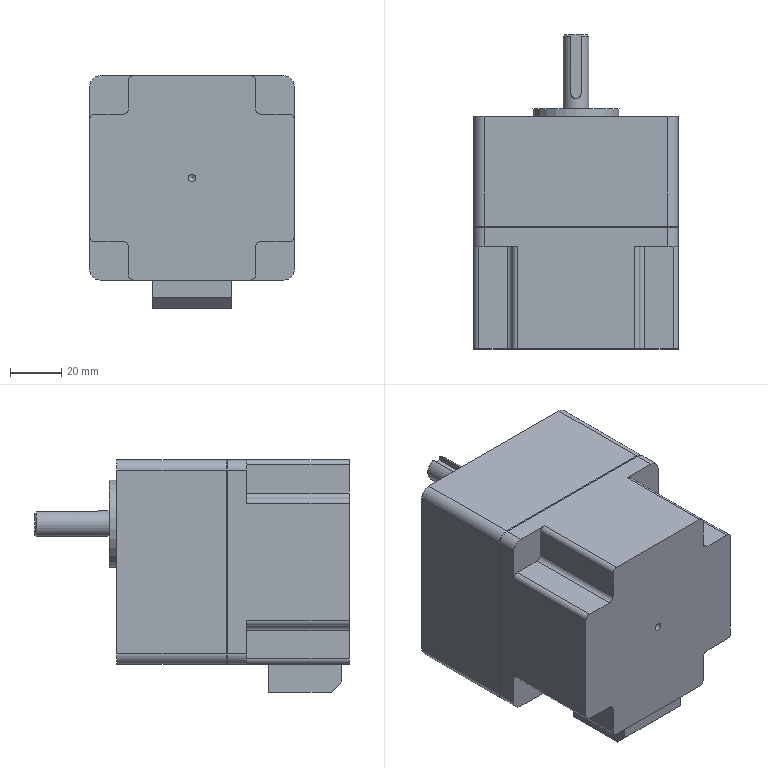Part | NX | features BREP 1 | 1 solid | 68 faces | box 80 x 123 x 91 mm | volume 559615 mm3 | plane 38 | cylinder 24 | cone 6 | commonest cylinder face diameters 4 x13 8 x8 3 x1 10 x1 34 x1